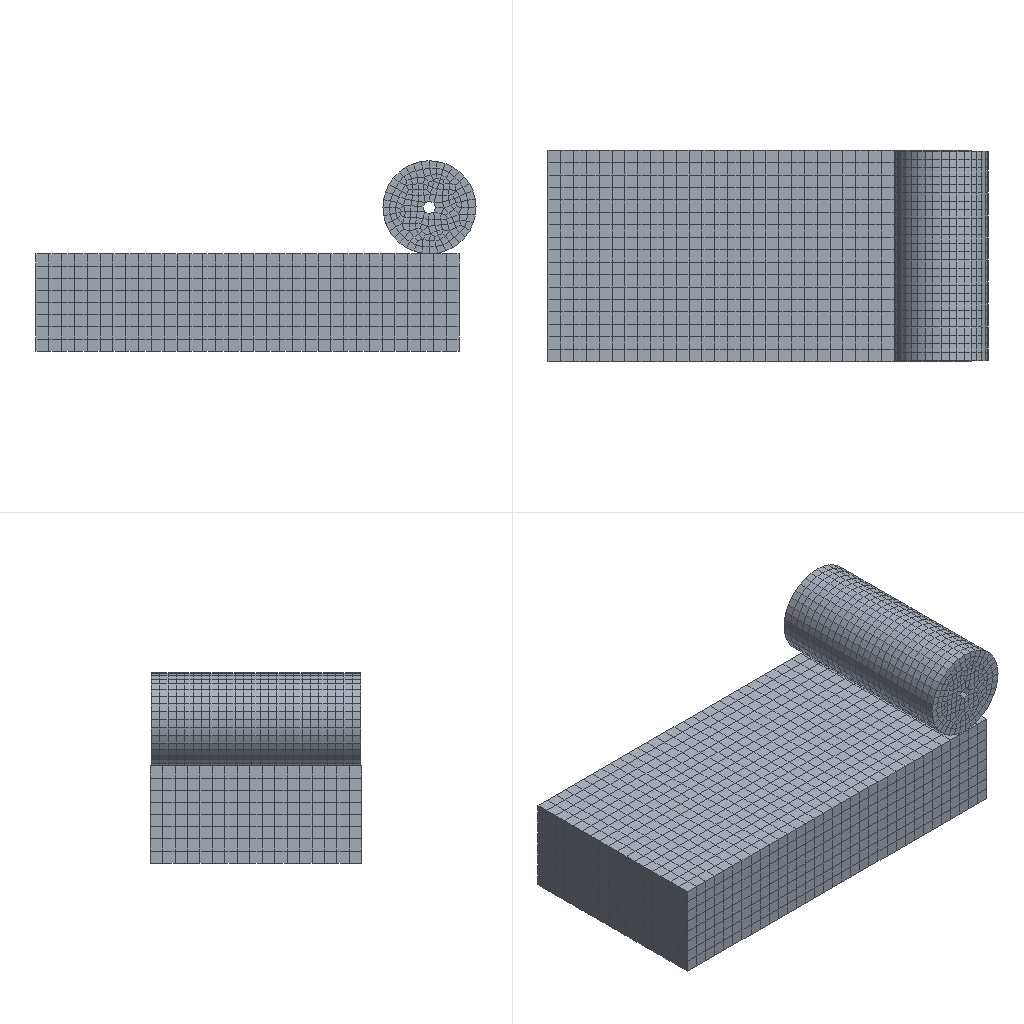Simulation study | abaqus
Set-up summary:
category,name,step,type,value,unit,region
solver,abaqus
solver,version,,,Abaqus/Explicit 2020
units,not stated in the deck,,not stated
analysis,deck,,dynamic temperature-displacement,dynamic temperature-displacement
load_step,Step-1,Step-1,dynamic temperature-displacement
load_step,requested,,,1
mesh,nodes,,,10604
mesh,elements,,,8838
element_type,C3D8RT,,solid,8838
load,load commands in deck,,count,2
bc,support commands in deck,,count,10
material,MATERIAL-1,,in results
check,setup vs results,,match,"per instance, exact: element labels, types and connectivity; labels of the nodes the elements use; coordinates of those nodes at SINGLE_PRECISION in 2 of 2 instance(s)"
Abaqus input file, long lists of numbers shortened:
*Heading
** Job name: Job-1 Model name: Model-1
** Generated by: Abaqus/CAE 2020
*Preprint, echo=NO, model=NO, history=NO, contact=NO
**
** PARTS
**
*Part, name=ban
*Node
      1,        -500.,        -500.,         230.
      2,        -500.,  -470.588,         230.
** (5506 more lines like these left out)
*Element, type=C3D8RT
   1,  163,  164,  182,  181,    1,    2,   20,   19
   2,  164,  165,  183,  182,    2,    3,   21,   20
** (4486 more lines like these left out)
*Nset, nset=Set-1, generate
    1,  5508,     1
*Elset, elset=Set-1, generate
    1,  4488,     1
** Section: Section-1
*Solid Section, elset=Set-1, material=Material-1
,
*End Part
**
*Part, name=gun
*Node
      1,   14.982, -0.7376,           0.
      2,   11.115,   10.072,           0.
** (5094 more lines like these left out)
*Element, type=C3D8RT
   1,  333,  286,  249,  299,  137,   90,   53,  103
   2,  242,  258,  197,  198,   46,   62,    1,    2
** (4348 more lines like these left out)
*Nset, nset=Set-3, generate
    1,  5096,     1
*Elset, elset=Set-3, generate
    1,  4350,     1
** Section: Section-1
*Solid Section, elset=Set-3, material=Material-1
,
*End Part
**
**
** ASSEMBLY
**
*Assembly, name=Assembly
**
*Instance, name=ban-1, part=ban
       -430.,           0.,        -345.
*End Instance
**
*Instance, name=gun-1, part=gun
          0.,         -2.5,          -5.
          0.,         -2.5,          -5., 1.,         -2.5,          -5., 90.
*End Instance
**
*Node
      1,           0.,        -250.,          -5.
*Nset, nset=Set-1, instance=gun-1
    1,    2,    3,    4,    5,    6,    7,    8,  197,  198,  199,  200,  201,  202,  203,  204
  393,  394,  395,  396,  397,  398,  399,  400,  589,  590,  591,  592,  593,  594,  595,  596
** (11 more lines like these left out)
*Elset, elset=Set-1, instance=gun-1
    2,    5,    6,   15,   19,   27,   31,   42,  176,  179,  180,  189,  193,  201,  205,  216
  350,  353,  354,  363,  367,  375,  379,  390,  524,  527,  528,  537,  541,  549,  553,  564
** (11 more lines like these left out)
*Nset, nset=Set-2, instance=ban-1
    1,    2,    3,    4,    5,    6,    7,    8,    9,   10,   11,   12,   13,   14,   15,   16
   17,   18,   19,   20,   21,   22,   23,   24,   25,   26,   27,   28,   29,   30,   31,   32
** (55 more lines like these left out)
*Elset, elset=Set-2, instance=ban-1
    1,    2,    3,    4,    5,    6,    7,    8,    9,   10,   11,   12,   13,   14,   15,   16
   17,   18,   19,   20,   21,   22,   23,   24,   25,   26,   27,   28,   29,   30,   31,   32
** (46 more lines like these left out)
*Nset, nset=Set-3, instance=ban-1, generate
   1,  162,    1
*Elset, elset=Set-3, instance=ban-1, generate
   1,  136,    1
*Nset, nset=Set-4, instance=gun-1
    1,    2,    3,    4,    5,    6,    7,    8,    9,   10,   11,   12,   13,   14,   15,   16
   17,   18,   19,   20,   21,   22,   23,   24,   25,   26,   27,   28,   29,   30,   31,   32
** (23 more lines like these left out)
*Elset, elset=Set-4, instance=gun-1
    1,    2,    3,    4,    5,    6,    7,    8,    9,   10,   11,   12,   13,   14,   15,   16
   17,   18,   19,   20,   21,   22,   23,   24,   25,   26,   27,   28,   29,   30,   31,   32
** (20 more lines like these left out)
*Nset, nset=Set-5, instance=gun-1
    1,    2,    3,    4,    5,    6,    7,    8,  197,  198,  199,  200,  201,  202,  203,  204
  393,  394,  395,  396,  397,  398,  399,  400,  589,  590,  591,  592,  593,  594,  595,  596
** (11 more lines like these left out)
*Elset, elset=Set-5, instance=gun-1
    2,    5,    6,   15,   19,   27,   31,   42,  176,  179,  180,  189,  193,  201,  205,  216
  350,  353,  354,  363,  367,  375,  379,  390,  524,  527,  528,  537,  541,  549,  553,  564
** (11 more lines like these left out)
*Nset, nset=Set-7
 1,
*Nset, nset=m_Set-6
 1,
*Elset, elset=_Surf-1_S5, internal, instance=ban-1
  120,  121,  122,  123,  124,  125,  126,  127,  128,  129,  130,  131,  132,  133,  134,  135
  136,  256,  257,  258,  259,  260,  261,  262,  263,  264,  265,  266,  267,  268,  269,  270
** (34 more lines like these left out)
*Surface, type=ELEMENT, name=Surf-1
_Surf-1_S5, S5
*Elset, elset=_m_Surf-2_S3, internal, instance=ban-1
    1,    2,    3,    4,    5,    6,    7,    8,    9,   10,   11,   12,   13,   14,   15,   16
   17,  137,  138,  139,  140,  141,  142,  143,  144,  145,  146,  147,  148,  149,  150,  151
** (34 more lines like these left out)
*Surface, type=ELEMENT, name=m_Surf-2
_m_Surf-2_S3, S3
*Elset, elset=_s_Surf-2_S5, internal, instance=gun-1
   10,   12,   14,   16,   18,   23,   29,   30,   33,   34,   38,   39,   41,   43,   46,   65
   67,   75,   78,   83,  184,  186,  188,  190,  192,  197,  203,  204,  207,  208,  212,  213
** (30 more lines like these left out)
*Elset, elset=_s_Surf-2_S3, internal, instance=gun-1
   25,   28,   32,   36,   40,   51,   53,   54,   56,   57,   58,   70,   76,   80,   84,   85
  199,  202,  206,  210,  214,  225,  227,  228,  230,  231,  232,  244,  250,  254,  258,  259
** (23 more lines like these left out)
*Surface, type=ELEMENT, name=s_Surf-2
_s_Surf-2_S5, S5
_s_Surf-2_S3, S3
*Elset, elset=_s_Surf-4_S5, internal, instance=gun-1
    2,    6,   27,  176,  180,  201,  350,  354,  375,  524,  528,  549,  698,  702,  723,  872
  876,  897, 1046, 1050, 1071, 1220, 1224, 1245, 1394, 1398, 1419, 1568, 1572, 1593, 1742, 1746
** (3 more lines like these left out)
*Elset, elset=_s_Surf-4_S6, internal, instance=gun-1
    5,   15,  179,  189,  353,  363,  527,  537,  701,  711,  875,  885, 1049, 1059, 1223, 1233
 1397, 1407, 1571, 1581, 1745, 1755, 1919, 1929, 2093, 2103, 2267, 2277, 2441, 2451, 2615, 2625
** (2 more lines like these left out)
*Elset, elset=_s_Surf-4_S3, internal, instance=gun-1, generate
   19,  4195,   174
*Elset, elset=_s_Surf-4_S4, internal, instance=gun-1
   31,   42,  205,  216,  379,  390,  553,  564,  727,  738,  901,  912, 1075, 1086, 1249, 1260
 1423, 1434, 1597, 1608, 1771, 1782, 1945, 1956, 2119, 2130, 2293, 2304, 2467, 2478, 2641, 2652
** (2 more lines like these left out)
*Surface, type=ELEMENT, name=s_Surf-4
_s_Surf-4_S5, S5
_s_Surf-4_S6, S6
_s_Surf-4_S4, S4
_s_Surf-4_S3, S3
** Constraint: Constraint-1
*Coupling, constraint name=Constraint-1, ref node=m_Set-6, surface=s_Surf-4
*Kinematic
*End Assembly
*Amplitude, name=Amp-1
             0.,              0.,              1.,              1.
**
** MATERIALS
**
*Material, name=Material-1
*Conductivity
30.,
*Density
 2.6e-09,
*Elastic
72000., 0.3
*Expansion
 1e-06,
*Specific Heat
 4e+08,
**
** INTERACTION PROPERTIES
**
*Surface Interaction, name=IntProp-1
*Friction
 0.5,
*Surface Behavior, pressure-overclosure=HARD
*Gap Conductance
 0.8,    0.
  0., 0.001
** ----------------------------------------------------------------
**
** STEP: Step-1
**
*Step, name=Step-1, nlgeom=YES
*Dynamic Temperature-displacement, Explicit
, 1.
*Bulk Viscosity
0.06, 1.2
** Mass Scaling: Semi-Automatic
**               Whole Model
*Fixed Mass Scaling, factor=500.
**
** BOUNDARY CONDITIONS
**
** Name: BC-1 Type: 位移/转角
*Boundary
Set-7, 1, 1
Set-7, 2, 2
Set-7, 3, 3
Set-7, 4, 4
Set-7, 6, 6
** Name: BC-2 Type: 位移/转角
*Boundary
Set-2, 2, 2
Set-2, 4, 4
Set-2, 5, 5
Set-2, 6, 6
** Name: BC-3 Type: 位移/转角
*Boundary, amplitude=Amp-1
Set-3, 1, 1, 900.
**
** LOADS
**
** Name: Load-1   Type: Pressure
*Dsload
Surf-1, P, 5.
**
** INTERACTIONS
**
** Interaction: Int-1
*Contact Pair, interaction=IntProp-1, mechanical constraint=KINEMATIC, cpset=Int-1
s_Surf-2, m_Surf-2
**
** OUTPUT REQUESTS
**
*Restart, write, number interval=1, time marks=NO
**
** FIELD OUTPUT: F-Output-1
**
*Output, field, number interval=50
*Node Output
CF, NT, RF, RFL, RM, RT, U, V
*Element Output, directions=YES
E, HFL, LE, MISES, MISESMAX, MISESONLY, PE, PEEQ, PEEQMAX, PEEQT, PEMAG, S, SF, SSAVG, TEMP, TSHR
VEEQ, YIELDPOT
*Contact Output
CDISP, CSTRESS
**
** HISTORY OUTPUT: H-Output-1
**
*Output, history, variable=PRESELECT, frequency=1
*End Step
Results summary:
result,step,Step-1,completed,increments=26280 time=1.0/1.0
result,analysis,,,"dynamic temperature-displacement, explict"
result,last_loadstep,,,1
result,primary field,,,"U, NT11"
result,reaction total,,FX,-11011027.801,model units
result,reaction total,,FY,-4243.544,model units
result,reaction total,,FZ,-5542166.5,model units